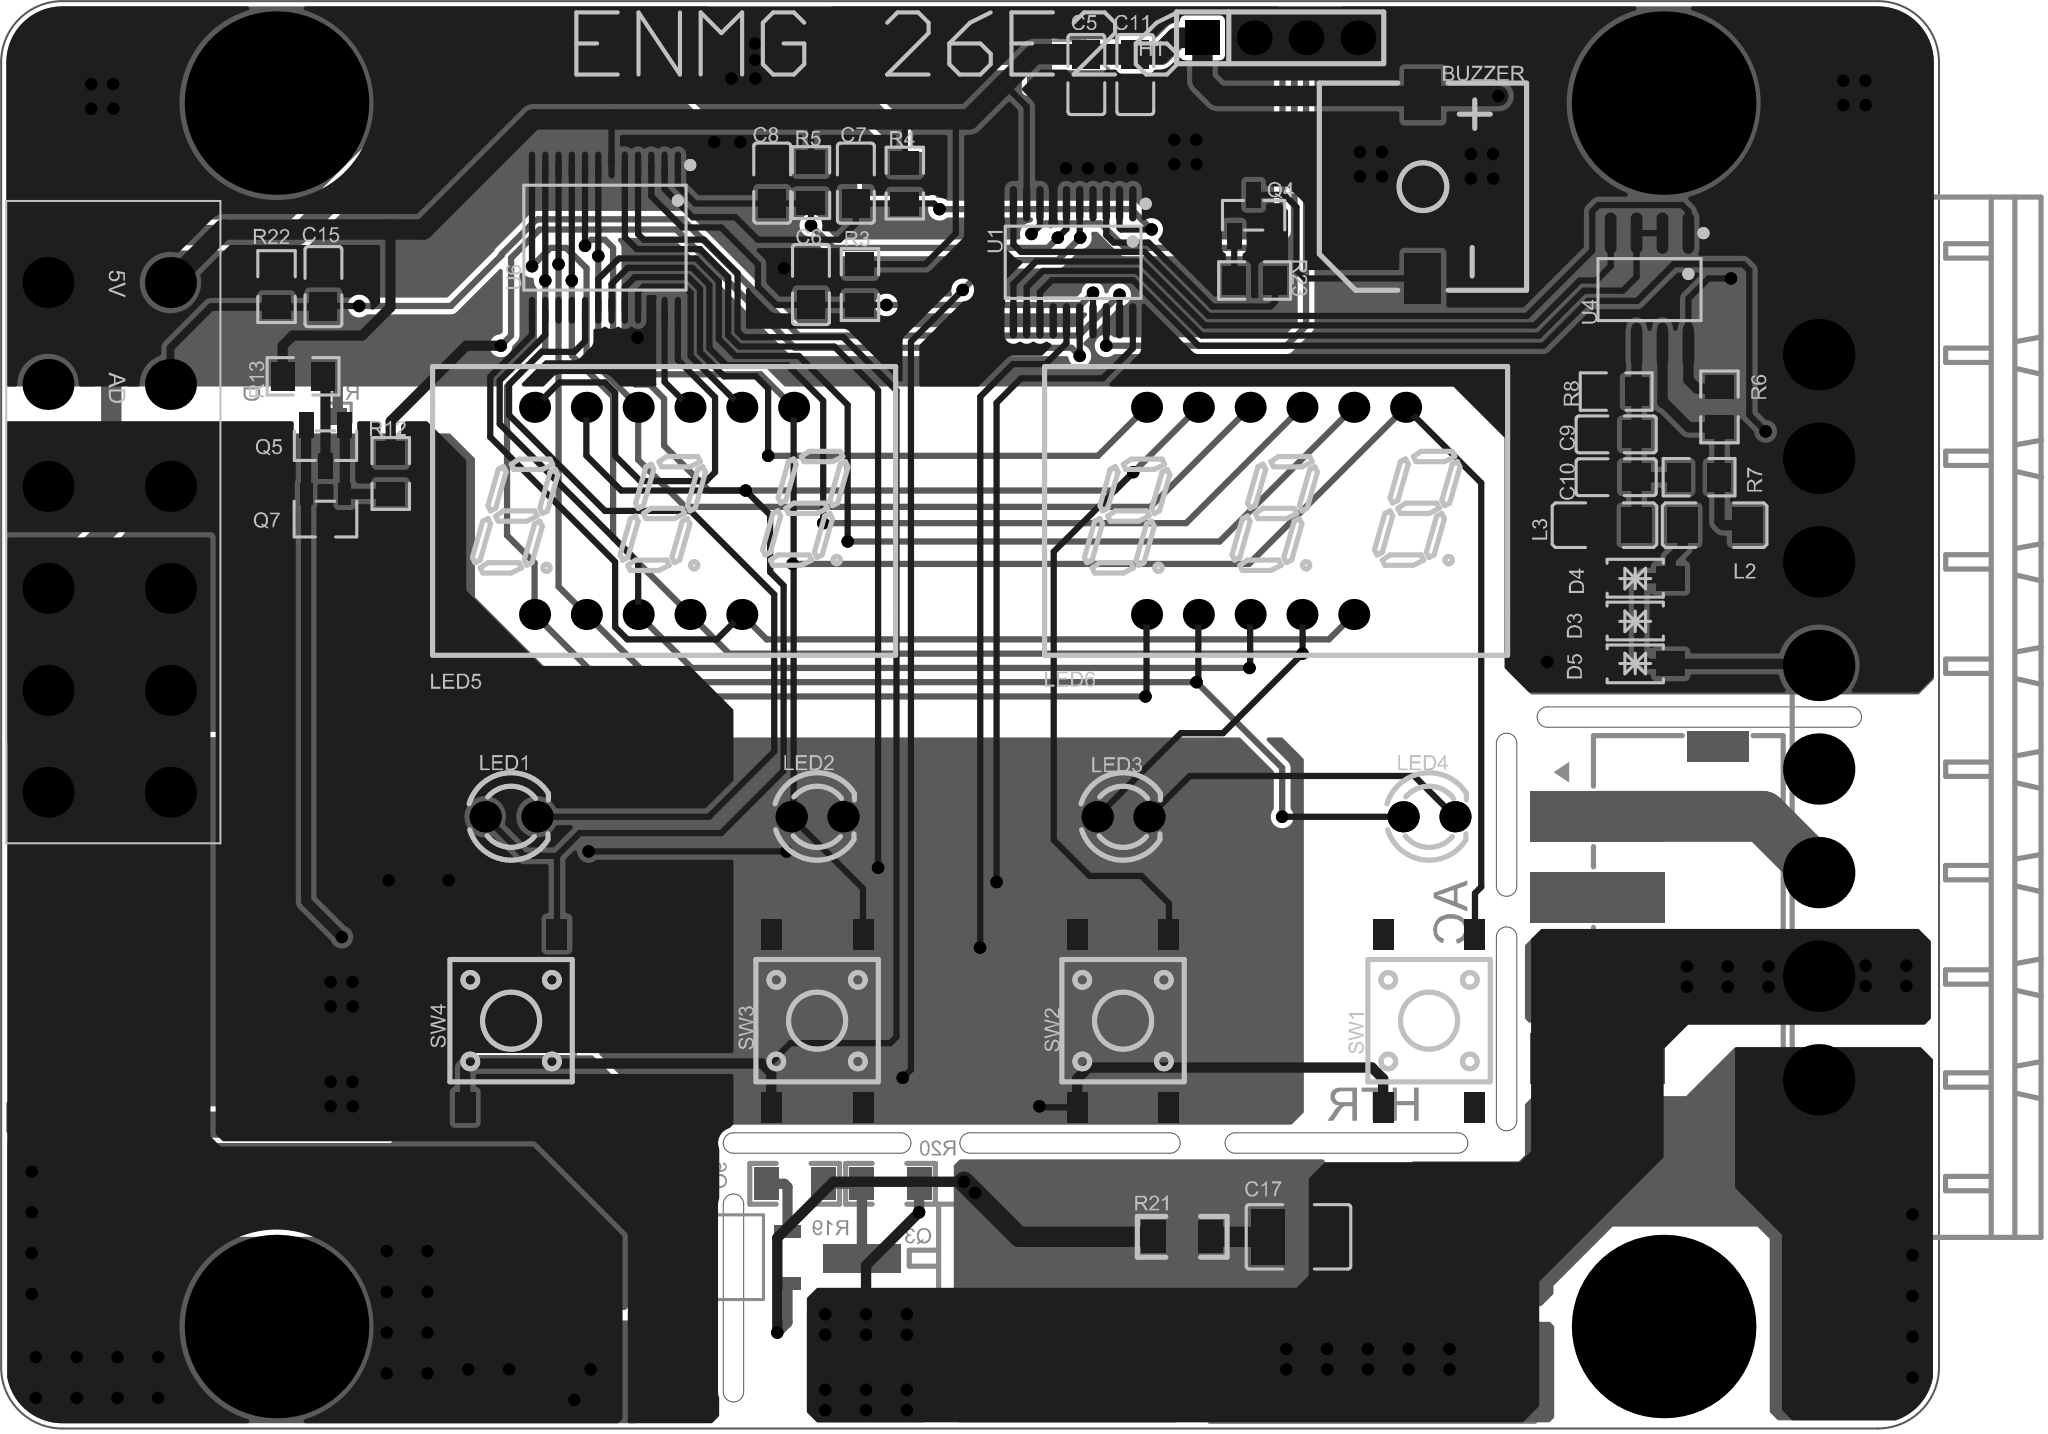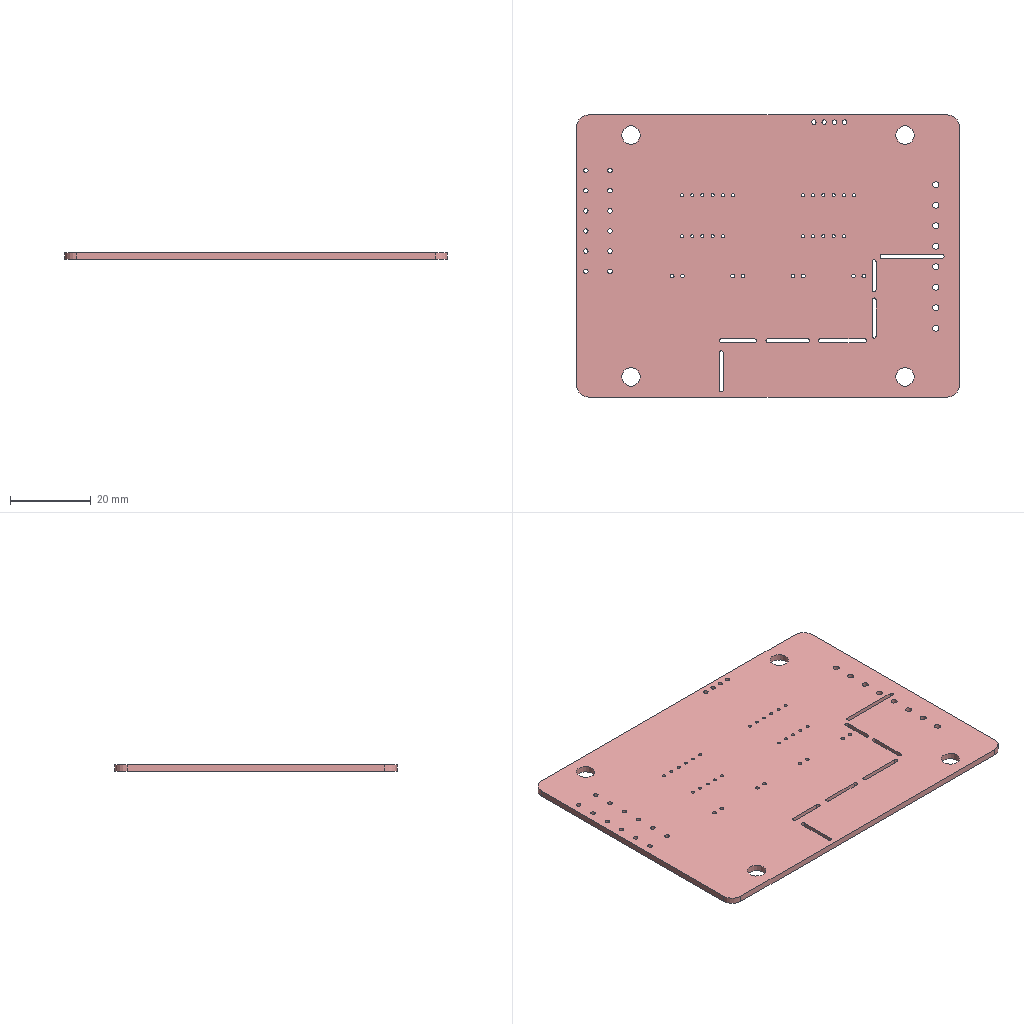Circuit board layout | Altium Designer | box 95 x 70 x 1.6 mm
Layer stack:
# Altium Designer layer stack of  (unit mm; dielectric type: 0 none, 1 core, 2 prepreg, 3 surface material)
index,name,kind,layer,copper_thickness_mm,dielectric_type,dielectric_thickness_mm,dielectric_material,dielectric_constant
0,Top Paste Mask Layer,other,,,,,,
1,Top Silkscreen Layer,other,,,,,,
2,Top Solder Mask Layer,dielectric,,,3,0.0102,,3.3
3,Top Layer,copper,Top Layer,0.0356,,,,
4,Dielectric1,dielectric,,,3,1.509,FR4,4.5
5,Bottom Layer,copper,Bottom Layer,0.0356,,,,
6,Bottom Solder Mask Layer,dielectric,,,3,0.0102,,3.3
7,Bottom Silkscreen Layer,other,,,,,,
8,Bottom Paste Mask Layer,other,,,,,,
# drill layer pairs: low layer,high layer
drill_pair,Top Layer,Bottom Layer
Part placement:
Designator,Comment,Layer,Footprint,Center-X(mm),Center-Y(mm),Rotation
C4,220uF,BottomLayer,CAP-SMD_BD6.3-L6.6-W6.6-FD,128.394,141.2,270
C1,220uF,BottomLayer,CAP-SMD_BD6.3-L6.6-W6.6-FD,105.514,141.2,270
H1,PZ254V-11-04P,TopLayer,HDR-TH_4P-P2.54-V-M,140.2,144.701,0
D2,SS34,BottomLayer,SMA_L4.3-W2.6-LS5.2-RD,116.23,141.671,270
U3,XL1509-5.0,BottomLayer,SOIC-8_L4.9-W3.9-P1.27-LS6.0-TR,111.823,141.13,180
C2,100nF,BottomLayer,C0805,100.907,142.87,270
C3,100nF,BottomLayer,C0805,133.101,142.9,90
C11,100nF,TopLayer,C0805,133.101,142.9,90
FAN,XH2.54-2P vertical SMD,BottomLayer,CONN-SMD_2P_A2501WV-S,100.7,82.3,90
FAN2,XH2.54-2P vertical SMD,BottomLayer,CONN-SMD_2P_A2501WV-S,82.099,86.1,90
L1,68uH,BottomLayer,IND-SMD_L7.1-W6.6_H5.0,121.389,140.957,270
BUZZER,2.7kHz,TopLayer,BUZ-SMD_L9.6-W9.6-LS10.0-R,147.201,137.4,90
C16,100nF,BottomLayer,C0805,111.295,104.029,270
C15,100nF,TopLayer,C0805,93.299,132.5,270
C9,100nF,TopLayer,C0805,156.672,125.252,0
C10,100nF,TopLayer,C0805,156.672,123.152,0
D5,SMF36CA,TopLayer,SOD-123_L2.7-W1.8-LS3.7-BI,157.607,113.998,180
D3,SMF36CA,TopLayer,SOD-123_L2.7-W1.8-LS3.7-BI,157.607,116.098,0
D4,SMF36CA,TopLayer,SOD-123_L2.7-W1.8-LS3.7-BI,157.607,118.199,0
L3,22uH,TopLayer,L1206,156.101,120.8,180
L2,22uH,TopLayer,L1206,161.501,120.8,180
LED1,3mmFIR,TopLayer,LED-TH_BD3.0-P2.54-FD,102.499,106.5,0
LED2,3mmFIR,TopLayer,LED-TH_BD3.0-P2.54-FD,117.5,106.5,0
LED3,3mmFIR,TopLayer,LED-TH_BD3.0-P2.54-FD,132.499,106.5,0
LED4,3mmFIR,TopLayer,LED-TH_BD3.0-P2.54-FD,147.5,106.5,0
LED5,SP420361N,TopLayer,LED-SEG-TH_SP420361N,110,121.501,270
LED6,SP420361N,TopLayer,LED-SEG-TH_SP420361N,140,121.501,270
Q1,NCE0140K2-VB,BottomLayer,TO-252-3_L6.6-W6.1-P4.58-LS10.1-BR,102.3,94.9,90
Q5,SS8050(RANGE:200-350),TopLayer,SOT-23-3_L2.9-W1.3-P1.90-LS2.4-BR,93.401,124.7,90
Q2,HYG025N06LS1B,BottomLayer,TO-263-2_L10.2-W8.7-P5.08-LS15.1-BR,88.5,98.1,0
Q4,SS8050(RANGE:200-350),TopLayer,SOT-23-3_L2.9-W1.3-P1.90-LS2.4-BR,138.9,136,270
R22,10kΩ,TopLayer,R0805,91.001,132.5,270
R9,10K,BottomLayer,R0805,111.15,98.75,270
R10,10kΩ,BottomLayer,R0805,109.05,98.75,270
R12,1kΩ,TopLayer,R0805,96.599,123.335,270
R6,47kΩ,TopLayer,R0805,161.737,126.599,90
R7,12kΩ,TopLayer,R0805,160.736,123.152,0
R8,47kΩ,TopLayer,R0805,156.672,127.353,0
R23,1kΩ,TopLayer,R0805,138.949,132.799,180
SW1,1TS005F-2500-5001,TopLayer,SW-SMD_4P-L6.0-W6.0-P4.50-LS9.0-H2.5,147.5,96.5,90
SW2,1TS005F-2500-5001,TopLayer,SW-SMD_4P-L6.0-W6.0-P4.50-LS9.0-H2.5,132.5,96.5,90
SW3,1TS005F-2500-5001,TopLayer,SW-SMD_4P-L6.0-W6.0-P4.50-LS9.0-H2.5,117.5,96.5,90
SW4,1TS005F-2500-5001,TopLayer,SW-SMD_4P-L6.0-W6.0-P4.50-LS9.0-H2.5,102.5,96.5,90
U1,LCM08F003,TopLayer,TSSOP-20_L6.5-W4.4-P0.65-LS6.4-BL,130.05,133.693,180
U4,MAX485ESA(UMW),TopLayer,SOP-8_L5.0-W4.0-P1.27-LS6.0-BL,158.308,132.353,180
C5,100nF,TopLayer,C0805,130.701,142.9,270
C6,100pF,TopLayer,C0805,117.201,132.599,270
C7,100pF,TopLayer,C0805,119.4,137.575,270
C8,100pF,TopLayer,C0805,115.301,137.575,270
R3,10kΩ,TopLayer,R0805,119.601,132.599,90
R4,10kΩ,TopLayer,R0805,121.801,137.575,90
R5,10kΩ,TopLayer,R0805,117.201,137.601,90
U6,TM1668-SSOP24-TA2108,TopLayer,SSOP-24_L8.1-W5.3-P0.65-LS7.8-BL,107.1,134.901,180
R11,1Ω,BottomLayer,R1206,109.057,104.508,270
R1,1kΩ,BottomLayer,R0805,162.301,126.399,90
R2,1kΩ,BottomLayer,R0805,162.301,130.2,90
C17,10nF,TopLayer,C1210,141.101,85.9,180
Q3,BTA216B-600D-JSM,BottomLayer,TO-263-3_L10.2-W9.2-P5.08-LS15.4-BR,125.1,82.301,180
R19,51Ω,BottomLayer,R0204,116.401,88.501,0
R20,150Ω,BottomLayer,R0204,121.1,88.501,0
R21,120Ω,TopLayer,R0204,135.4,85.9,180
U5,ELM3083(TA)-V,BottomLayer,SOP-4_L4.4-W4.0-P2.54-LS7.0-TL,112.9,84.9,0
CN1,KF2EDGRM-5.08-8P,BottomLayer,CONN-TH_8P-P5.08_KF2EDGRM-5.08-8P,166.601,111.382,270
Q6,SS8050(RANGE:200-350),BottomLayer,SOT-23-3_L2.9-W1.3-P1.90-LS2.4-BR,110.5,89,90
R16,1kΩ,BottomLayer,R0805,111.6,92.7,270
R17,10kΩ,BottomLayer,R0805,109.499,92.7,90
R18,2.2kΩ,BottomLayer,R0805,111.501,79.099,270
HTR,VH3.96-3P,BottomLayer,CONN-SMD_3P-P3.96_HCTL_HC-VH-3ALT,144.7,83,180
AC,BX-VH3.96-5PLT,BottomLayer,CONN-SMD_5P-P3.96_BX-VH3.96-5PLT,158.701,98.6,270
D1,M7,BottomLayer,SMA_L4.4-W2.8-LS5.4-RD,98.3,141.3,270
Q7,LBC807-25LT1G,TopLayer,SOT-23-3_L2.9-W1.6-P1.90-LS2.8-BR,93.401,121.1,90
C12,1nF,BottomLayer,C0805,155.001,128.2,270
D6,SS34,BottomLayer,SMA_L4.3-W2.6-LS5.2-RD,90.099,110.5,270
R13,47Ω,TopLayer,R0805,92.3,128.1,180
D7,SS34,BottomLayer,SMA_L4.3-W2.6-LS5.2-RD,107.201,81.699,90
R14,10K,BottomLayer,R0603,94,125.4,90
Pad and via stacks:
# Altium Designer via and pad stacks of  (unit mm). Each distinct definition once, with the count of objects using it.
# via: kind,start_layer,end_layer,hole_mm,diameter_mm,mode(0 simple;1 top-mid-bottom;2 full stack),diameter_per_layer,count,example_net
# pad: kind,layer,hole_mm,hole_type(0 round;1 square;2 slot),plating,top_size,top_shape(1 round;2 rect;3 octagon;9 rounded rect),mid_size,bottom_size,mode,footprint,size_per_layer,count,example
pad,Multi-Layer,4.6,0,plated,8.999x8.999,1,5.001x5.001,7x7,1,,,4,1
pad,Multi-Layer,1.1,0,plated,1.699x1.699,2,1.699x1.699,1.699x1.699,0,HDR-TH_4P-P2.54-V-M,,1,H1.1
pad,Multi-Layer,1.1,0,plated,1.699x1.699,1,1.699x1.699,1.699x1.699,0,HDR-TH_4P-P2.54-V-M,,3,H1.2
pad,Multi-Layer,0.9144,0,plated,1.524x1.524,1,1.524x1.524,1.524x1.524,0,LED-TH_BD3.0-P2.54-FD,,8,LED1.1
pad,Multi-Layer,0.762,0,plated,1.001x1.001,1,1.001x1.001,1.524x1.524,1,LED-SEG-TH_SP420361N,,22,LED5.1
pad,Multi-Layer,1.501,0,plated,3.5x3.5,1,2.499x2.499,2.499x2.499,1,CONN-TH_8P-P5.08_KF2EDGRM-5.08-8P,,8,CN1.1
pad,Multi-Layer,1.1,0,plated,2.499x2.499,1,1.3x1.3,1.501x1.501,1,,,10,0
pad,Multi-Layer,1.1,0,plated,2.499x2.499,1,1.3x1.3,2.499x2.499,1,,,2,0
pad,Bottom Layer,0,0,plated,3.5x1.199,2,3.5x1.199,3.5x1.199,0,CAP-SMD_BD6.3-L6.6-W6.6-FD,,4,C4.1
pad,Bottom Layer,0,0,plated,1.999x1.999,2,1.999x1.999,1.999x1.999,0,SMA_L4.3-W2.6-LS5.2-RD,,6,D2.2
pad,Bottom Layer,0,0,plated,0.5994x1.519,1,0.5994x1.519,0.5994x1.519,0,SOIC-8_L4.9-W3.9-P1.27-LS6.0-TR,,8,U3.5
pad,Bottom Layer,0,0,plated,1.41x1.349,2,1.41x1.349,1.41x1.349,0,C0805,,8,C2.2
pad,Bottom Layer,0,0,plated,1.1x2.499,2,1.1x2.499,1.1x2.499,0,CONN-SMD_2P_A2501WV-S,,4,FAN.4
pad,Bottom Layer,0,0,plated,1.199x5.7,2,1.199x5.7,1.199x5.7,0,CONN-SMD_2P_A2501WV-S,,4,FAN.1
pad,Bottom Layer,0,0,plated,2.149x3.32,2,2.149x3.32,2.149x3.32,0,IND-SMD_L7.1-W6.6_H5.0,,2,L1.2
pad,Bottom Layer,0,0,plated,6.5x6,2,6.5x6,6.5x6,0,TO-252-3_L6.6-W6.1-P4.58-LS10.1-BR,,1,Q1.3
pad,Bottom Layer,0,0,plated,3x1.6,2,3x1.6,3x1.6,0,TO-252-3_L6.6-W6.1-P4.58-LS10.1-BR,,2,Q1.1
pad,Bottom Layer,0,0,plated,8.839x11.001,2,8.839x11.001,8.839x11.001,0,TO-263-2_L10.2-W8.7-P5.08-LS15.1-BR,,1,Q2.4
pad,Bottom Layer,0,0,plated,3.81x1.999,2,3.81x1.999,3.81x1.999,0,TO-263-2_L10.2-W8.7-P5.08-LS15.1-BR,,2,Q2.3
pad,Bottom Layer,0,0,plated,1.133x1.377,2,1.133x1.377,1.133x1.377,0,R0805,,14,R9.2
pad,Bottom Layer,0,0,plated,1.206x1.702,2,1.206x1.702,1.206x1.702,0,R1206,,2,R11.2
pad,Bottom Layer,0,0,plated,3.8x1.399,2,3.8x1.399,3.8x1.399,0,TO-263-3_L10.2-W9.2-P5.08-LS15.4-BR,,2,Q3.1
pad,Bottom Layer,0,0,plated,8.801x10.701,2,8.801x10.701,8.801x10.701,0,TO-263-3_L10.2-W9.2-P5.08-LS15.4-BR,,1,Q3.2
pad,Bottom Layer,0,0,plated,1.199x1.6,2,1.199x1.6,1.199x1.6,0,R0204,,4,R19.2
pad,Bottom Layer,0,0,plated,0.5944x1.3,2,0.5944x1.3,0.5944x1.3,0,SOP-4_L4.4-W4.0-P2.54-LS7.0-TL,,4,U5.1
pad,Bottom Layer,0,0,plated,1.25x0.701,2,1.25x0.701,1.25x0.701,0,SOT-23-3_L2.9-W1.3-P1.90-LS2.4-BR,,3,Q6.1
pad,Bottom Layer,0,0,plated,2.499x7,2,2.499x7,2.499x7,0,CONN-SMD_3P-P3.96_HCTL_HC-VH-3ALT,,3,HTR.1
pad,Bottom Layer,0,0,plated,1.501x3,2,1.501x3,1.501x3,0,CONN-SMD_3P-P3.96_HCTL_HC-VH-3ALT,,2,HTR.4
pad,Bottom Layer,0,0,plated,2.499x6.599,2,2.499x6.599,2.499x6.599,0,CONN-SMD_5P-P3.96_BX-VH3.96-5PLT,,5,AC.1
pad,Bottom Layer,0,0,plated,1.501x3,2,1.501x3,1.501x3,0,CONN-SMD_5P-P3.96_BX-VH3.96-5PLT,,2,AC.7
pad,Bottom Layer,0,0,plated,2.047x1.621,2,2.047x1.621,2.047x1.621,0,SMA_L4.4-W2.8-LS5.4-RD,,2,D1.2
pad,Bottom Layer,0,0,plated,0.8077x0.8636,2,0.8077x0.8636,0.8077x0.8636,0,R0603,,2,R14.2
pad,Top Layer,0,0,plated,1.41x1.349,2,1.41x1.349,1.41x1.349,0,C0805,,16,C11.2
pad,Top Layer,0,0,plated,2.499x1.801,2,2.499x1.801,2.499x1.801,0,BUZ-SMD_L9.6-W9.6-LS10.0-R,,2,BUZZER.1
pad,Top Layer,0,0,plated,1.399x1.199,2,1.399x1.199,1.399x1.199,0,SOD-123_L2.7-W1.8-LS3.7-BI,,6,D5.2
pad,Top Layer,0,0,plated,1.486x1.727,2,1.486x1.727,1.486x1.727,0,L1206,,4,L3.2
pad,Top Layer,0,0,plated,1.25x0.701,2,1.25x0.701,1.25x0.701,0,SOT-23-3_L2.9-W1.3-P1.90-LS2.4-BR,,6,Q5.1
pad,Top Layer,0,0,plated,1.133x1.377,2,1.133x1.377,1.133x1.377,0,R0805,,20,R22.2
pad,Top Layer,0,0,plated,1.501x1.001,2,1.501x1.001,1.501x1.001,0,SW-SMD_4P-L6.0-W6.0-P4.50-LS9.0-H2.5,,16,SW1.1
pad,Top Layer,0,0,plated,0.3632x1.742,1,0.3632x1.742,0.3632x1.742,0,TSSOP-20_L6.5-W4.4-P0.65-LS6.4-BL,,20,U1.1
pad,Top Layer,0,0,plated,0.574x2.034,1,0.574x2.034,0.574x2.034,0,SOP-8_L5.0-W4.0-P1.27-LS6.0-BL,,8,U4.1
pad,Top Layer,0,0,plated,0.3073x1.323,1,0.3073x1.323,0.3073x1.323,0,SSOP-24_L8.1-W5.3-P0.65-LS7.8-BL,,24,U6.1
pad,Top Layer,0,0,plated,1.636x2.7,2,1.636x2.7,1.636x2.7,0,C1210,,2,C17.2
pad,Top Layer,0,0,plated,1.199x1.6,2,1.199x1.6,1.199x1.6,0,R0204,,2,R21.2
pad,Top Layer,0,0,plated,1.069x0.5994,2,1.069x0.5994,1.069x0.5994,0,SOT-23-3_L2.9-W1.6-P1.90-LS2.8-BR,,3,Q7.1
via,Top Layer,Bottom Layer,0.3048,0.6096,0,,150,C
Copper pours:
name,layer,net,type(0 solid;1 hatched;2 none)
Bottom Layer-PL,Bottom Layer,PL,0
Bottom Layer-N,Bottom Layer,N,0
Bottom Layer-L,Bottom Layer,L,0
Bottom Layer-HTR1,Bottom Layer,HTR1,0
Bottom Layer-N 1,Bottom Layer,N,0
Bottom Layer-N 2,Bottom Layer,N,0
Bottom Layer-VCC,Bottom Layer,VCC,0
Bottom Layer-FAN1,Bottom Layer,FAN1,0
Bottom Layer-GND1,Bottom Layer,GND1,0
Bottom Layer-GND,Bottom Layer,GND,0
Top Layer-VCC,Top Layer,VCC,0
Top Layer-N,Top Layer,N,0
Top Layer-L,Top Layer,L,0
Top Layer-VCC 1,Top Layer,VCC,0
Top Layer-GND1,Top Layer,GND1,0
Top Layer-GND,Top Layer,GND,0
Design rules, without the lines most boards share:
# Altium Designer design rules of  (exported by Altium Designer, unit mm)
# columns: name | kind | enabled | priority | scope1 | scope2 | descriptor | typed fields (field=value)
HoleToHoleClearance | 52 | enabled | 1 | All | All | Hole To Hole Clearance (Gap=10mil) (All),(All) | gap=0.254
copperThickness1oz | 0 | enabled | 2 | All | All | Clearance Constraint (Gap=7mil) (All),(All) | gap=0.1778
copperThickness2oz | 0 | enabled | 1 | All | All | Clearance Constraint (Gap=7mil) (All),(All) | gap=0.1778
copperThickness2oz_1 | 63 | enabled | 1 | All | All | Board Clearance Constraint (Gap=0mil) (All) |
Plane_innerPlane | 0 | enabled | 3 | All | All | Clearance Constraint (Gap=7mil) (All),(All) | gap=0.1778
Plane_innerPlane_1 | 63 | enabled | 3 | All | All | Board Clearance Constraint (Gap=0mil) (All) |
Copper_copperRegion | 0 | enabled | 5 | All | All | Clearance Constraint (Gap=7mil) (All),(All) | gap=0.1778
Copper_copperRegion_1 | 63 | enabled | 5 | All | All | Board Clearance Constraint (Gap=0mil) (All) |
otherClearance | 0 | enabled | 4 | All | All | Clearance Constraint (Gap=7mil) (All),(All) | gap=0.1778
otherClearance_1 | 63 | enabled | 4 | All | All | Board Clearance Constraint (Gap=0mil) (All) |
copperThickness1oz_2 | 2 | enabled | 1 | All | All | Width Constraint (Min=5mil) (Max=100mil) (Preferred=10mil) (All) |
copperThickness2oz_2 | 2 | enabled | 2 | All | All | Width Constraint (Min=8mil) (Max=100mil) (Preferred=10mil) (All) |
trackWidth1 | 2 | enabled | 3 | All | All | Width Constraint (Min=5mil) (Max=100mil) (Preferred=30mil) (All) |
viaSize | 11 | enabled | 1 | All | All | Routing Via (MinHoleWidth=11.811mil) (MaxHoleWidth=248.031mil) (PreferredHoleWidth=12.008mil) (MinWidth=11.811mil) (MaxWidth=248.031mil) (PreferedWidth=12.008mil) (All) | via_min_hole=0.3 via_max_hole=6.3 via_preferred_diameter=0.305 via_preferred_hole=0.305
copperRegion | 20 | enabled | 1 | All | All | Polygon Connect Rule(Direct Connect )(Conductor Width=10mil) (Relief Angle=90 Angle) (Entries=4) (Air Gap Width=10mil) (All),(All) | connect_style(0=relief,1=direct,2=none)=1 relief_conductor_width=0.254 relief_entries=4